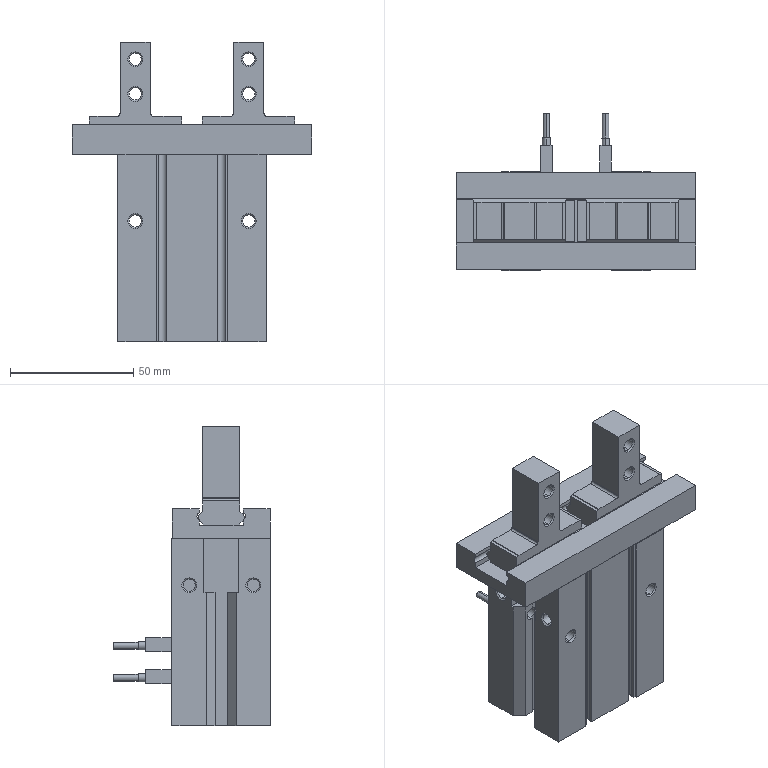Part | SolidWorks | features AEMSimFeature 1, MirrorCompFeat 1, ReferencePattern 1 | 5 solids | 313 faces | box 97 x 63.7 x 121.5 mm | volume 211309 mm3 | plane 191 | cylinder 80 | cone 42 | commonest cylinder face diameters 4.917 x24 4 x14 5.1 x8 2.1 x6 1.6 x4 2.5 x4